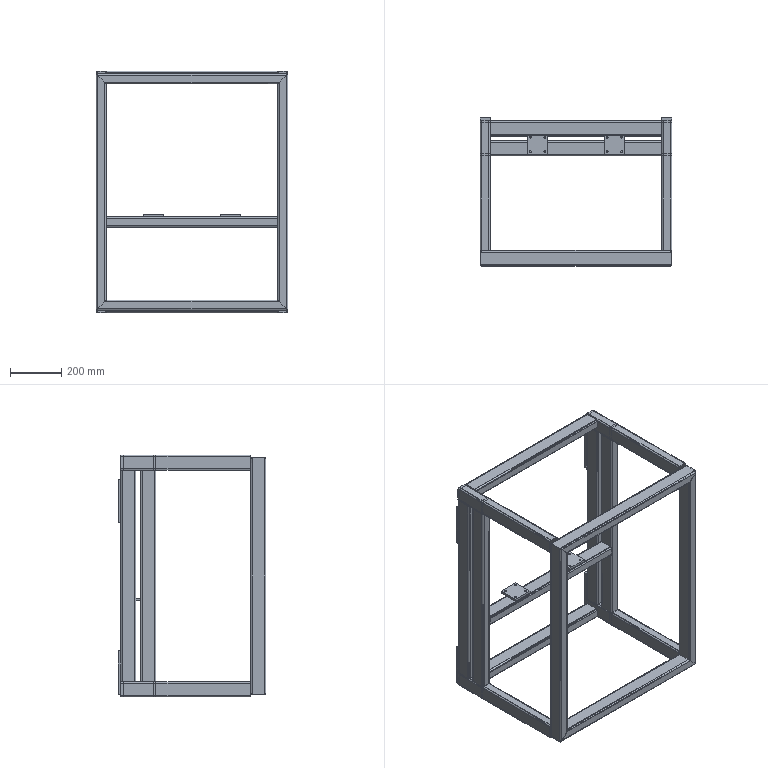Part | STEP file | 33 solids | 522 faces | box 750 x 578 x 945 mm | volume 6599392 mm3 | plane 274 | cylinder 248 | commonest cylinder face diameters 12.8 x108 6.4 x76 10.2 x32 6.8 x24 16 x8